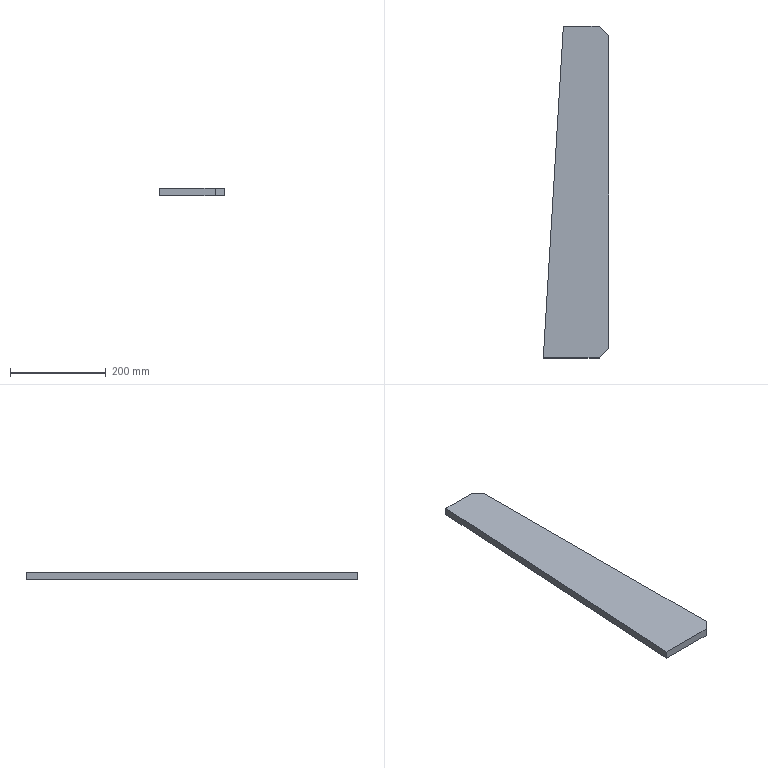Part | SolidWorks | features Chamfer 1, Extrusion 1 | 1 solid | 8 faces | box 137 x 695 x 16 mm | volume 1283520 mm3 | plane 8
STEP:
#1=CARTESIAN_POINT('',(0.,0.,-8.));
#2=VERTEX_POINT('',#1);
#3=CARTESIAN_POINT('',(117.,0.,-8.));
#4=VERTEX_POINT('',#3);
#5=CARTESIAN_POINT('',(137.,0.,-8.));
#6=DIRECTION('',(1.,0.,0.));
#7=VECTOR('',#6,1000.);
#8=LINE('',#5,#7);
#9=EDGE_CURVE('',#2,#4,#8,.T.);
#10=ORIENTED_EDGE('',*,*,#9,.T.);
#11=CARTESIAN_POINT('',(117.,0.,8.));
#12=VERTEX_POINT('',#11);
#13=CARTESIAN_POINT('',(117.,0.,8.));
#14=DIRECTION('',(0.,0.,1.));
#15=VECTOR('',#14,1000.);
#16=LINE('',#13,#15);
#17=EDGE_CURVE('',#4,#12,#16,.T.);
#18=ORIENTED_EDGE('',*,*,#17,.T.);
#19=CARTESIAN_POINT('',(0.,0.,8.));
#20=VERTEX_POINT('',#19);
#21=CARTESIAN_POINT('',(137.,0.,8.));
#22=DIRECTION('',(1.,0.,0.));
#23=VECTOR('',#22,1000.);
#24=LINE('',#21,#23);
#25=EDGE_CURVE('',#20,#12,#24,.T.);
#26=ORIENTED_EDGE('',*,*,#25,.F.);
#27=CARTESIAN_POINT('',(0.,0.,8.));
#28=DIRECTION('',(0.,0.,-1.));
#29=VECTOR('',#28,1000.);
#30=LINE('',#27,#29);
#31=EDGE_CURVE('',#20,#2,#30,.T.);
#32=ORIENTED_EDGE('',*,*,#31,.T.);
#33=EDGE_LOOP('',(#10,#18,#26,#32));
#34=FACE_OUTER_BOUND('',#33,.T.);
#35=CARTESIAN_POINT('',(137.,0.,8.));
#36=DIRECTION('',(0.,1.,0.));
#37=DIRECTION('',(0.,0.,1.));
#38=AXIS2_PLACEMENT_3D('',#35,#36,#37);
#39=PLANE('',#38);
#40=ADVANCED_FACE('',(#34),#39,.F.);
#41=CARTESIAN_POINT('',(137.,20.,8.));
#42=VERTEX_POINT('',#41);
#43=CARTESIAN_POINT('',(137.,675.,8.));
#44=VERTEX_POINT('',#43);
#45=CARTESIAN_POINT('',(137.,695.,8.));
#46=DIRECTION('',(0.,1.,0.));
#47=VECTOR('',#46,1000.);
#48=LINE('',#45,#47);
#49=EDGE_CURVE('',#42,#44,#48,.T.);
#50=ORIENTED_EDGE('',*,*,#49,.F.);
#51=CARTESIAN_POINT('',(137.,20.,-8.));
#52=VERTEX_POINT('',#51);
#53=CARTESIAN_POINT('',(137.,20.,8.));
#54=DIRECTION('',(0.,0.,-1.));
#55=VECTOR('',#54,1000.);
#56=LINE('',#53,#55);
#57=EDGE_CURVE('',#42,#52,#56,.T.);
#58=ORIENTED_EDGE('',*,*,#57,.T.);
#59=CARTESIAN_POINT('',(137.,675.,-8.));
#60=VERTEX_POINT('',#59);
#61=CARTESIAN_POINT('',(137.,695.,-8.));
#62=DIRECTION('',(0.,1.,0.));
#63=VECTOR('',#62,1000.);
#64=LINE('',#61,#63);
#65=EDGE_CURVE('',#52,#60,#64,.T.);
#66=ORIENTED_EDGE('',*,*,#65,.T.);
#67=CARTESIAN_POINT('',(137.,675.,8.));
#68=DIRECTION('',(0.,0.,1.));
#69=VECTOR('',#68,1000.);
#70=LINE('',#67,#69);
#71=EDGE_CURVE('',#60,#44,#70,.T.);
#72=ORIENTED_EDGE('',*,*,#71,.T.);
#73=EDGE_LOOP('',(#50,#58,#66,#72));
#74=FACE_OUTER_BOUND('',#73,.T.);
#75=CARTESIAN_POINT('',(137.,695.,8.));
#76=DIRECTION('',(-1.,0.,0.));
#77=DIRECTION('',(0.,-1.,0.));
#78=AXIS2_PLACEMENT_3D('',#75,#76,#77);
#79=PLANE('',#78);
#80=ADVANCED_FACE('',(#74),#79,.F.);
#81=CARTESIAN_POINT('',(117.,695.,8.));
#82=VERTEX_POINT('',#81);
#83=CARTESIAN_POINT('',(42.,695.,8.));
#84=VERTEX_POINT('',#83);
#85=CARTESIAN_POINT('',(42.,695.,8.));
#86=DIRECTION('',(-1.,0.,0.));
#87=VECTOR('',#86,1000.);
#88=LINE('',#85,#87);
#89=EDGE_CURVE('',#82,#84,#88,.T.);
#90=ORIENTED_EDGE('',*,*,#89,.F.);
#91=CARTESIAN_POINT('',(117.,695.,-8.));
#92=VERTEX_POINT('',#91);
#93=CARTESIAN_POINT('',(117.,695.,8.));
#94=DIRECTION('',(0.,0.,-1.));
#95=VECTOR('',#94,1000.);
#96=LINE('',#93,#95);
#97=EDGE_CURVE('',#82,#92,#96,.T.);
#98=ORIENTED_EDGE('',*,*,#97,.T.);
#99=CARTESIAN_POINT('',(42.,695.,-8.));
#100=VERTEX_POINT('',#99);
#101=CARTESIAN_POINT('',(42.,695.,-8.));
#102=DIRECTION('',(-1.,0.,0.));
#103=VECTOR('',#102,1000.);
#104=LINE('',#101,#103);
#105=EDGE_CURVE('',#92,#100,#104,.T.);
#106=ORIENTED_EDGE('',*,*,#105,.T.);
#107=CARTESIAN_POINT('',(42.,695.,8.));
#108=DIRECTION('',(0.,0.,-1.));
#109=VECTOR('',#108,1000.);
#110=LINE('',#107,#109);
#111=EDGE_CURVE('',#84,#100,#110,.T.);
#112=ORIENTED_EDGE('',*,*,#111,.F.);
#113=EDGE_LOOP('',(#90,#98,#106,#112));
#114=FACE_OUTER_BOUND('',#113,.T.);
#115=CARTESIAN_POINT('',(42.,695.,8.));
#116=DIRECTION('',(0.,-1.,0.));
#117=DIRECTION('',(0.,0.,-1.));
#118=AXIS2_PLACEMENT_3D('',#115,#116,#117);
#119=PLANE('',#118);
#120=ADVANCED_FACE('',(#114),#119,.F.);
#121=CARTESIAN_POINT('',(0.,0.,-8.));
#122=DIRECTION('',(-0.06032,-0.9982,0.));
#123=VECTOR('',#122,1000.);
#124=LINE('',#121,#123);
#125=EDGE_CURVE('',#100,#2,#124,.T.);
#126=ORIENTED_EDGE('',*,*,#125,.T.);
#127=ORIENTED_EDGE('',*,*,#31,.F.);
#128=CARTESIAN_POINT('',(0.,0.,8.));
#129=DIRECTION('',(-0.06032,-0.9982,0.));
#130=VECTOR('',#129,1000.);
#131=LINE('',#128,#130);
#132=EDGE_CURVE('',#84,#20,#131,.T.);
#133=ORIENTED_EDGE('',*,*,#132,.F.);
#134=ORIENTED_EDGE('',*,*,#111,.T.);
#135=EDGE_LOOP('',(#126,#127,#133,#134));
#136=FACE_OUTER_BOUND('',#135,.T.);
#137=CARTESIAN_POINT('',(0.,0.,8.));
#138=DIRECTION('',(0.9982,-0.06032,0.));
#139=DIRECTION('',(0.06032,0.9982,0.));
#140=AXIS2_PLACEMENT_3D('',#137,#138,#139);
#141=PLANE('',#140);
#142=ADVANCED_FACE('',(#136),#141,.F.);
#143=ORIENTED_EDGE('',*,*,#25,.T.);
#144=CARTESIAN_POINT('',(58.5,-58.5,8.));
#145=DIRECTION('',(0.7071,0.7071,0.));
#146=VECTOR('',#145,1000.);
#147=LINE('',#144,#146);
#148=EDGE_CURVE('',#12,#42,#147,.T.);
#149=ORIENTED_EDGE('',*,*,#148,.T.);
#150=ORIENTED_EDGE('',*,*,#49,.T.);
#151=CARTESIAN_POINT('',(406.,406.,8.));
#152=DIRECTION('',(-0.7071,0.7071,0.));
#153=VECTOR('',#152,1000.);
#154=LINE('',#151,#153);
#155=EDGE_CURVE('',#44,#82,#154,.T.);
#156=ORIENTED_EDGE('',*,*,#155,.T.);
#157=ORIENTED_EDGE('',*,*,#89,.T.);
#158=ORIENTED_EDGE('',*,*,#132,.T.);
#159=EDGE_LOOP('',(#143,#149,#150,#156,#157,#158));
#160=FACE_OUTER_BOUND('',#159,.T.);
#161=CARTESIAN_POINT('',(0.,0.,8.));
#162=DIRECTION('',(0.,0.,1.));
#163=DIRECTION('',(1.,0.,0.));
#164=AXIS2_PLACEMENT_3D('',#161,#162,#163);
#165=PLANE('',#164);
#166=ADVANCED_FACE('',(#160),#165,.T.);
#167=ORIENTED_EDGE('',*,*,#65,.F.);
#168=CARTESIAN_POINT('',(137.,20.,-8.));
#169=DIRECTION('',(-0.7071,-0.7071,0.));
#170=VECTOR('',#169,1000.);
#171=LINE('',#168,#170);
#172=EDGE_CURVE('',#52,#4,#171,.T.);
#173=ORIENTED_EDGE('',*,*,#172,.T.);
#174=ORIENTED_EDGE('',*,*,#9,.F.);
#175=ORIENTED_EDGE('',*,*,#125,.F.);
#176=ORIENTED_EDGE('',*,*,#105,.F.);
#177=CARTESIAN_POINT('',(117.,695.,-8.));
#178=DIRECTION('',(0.7071,-0.7071,0.));
#179=VECTOR('',#178,1000.);
#180=LINE('',#177,#179);
#181=EDGE_CURVE('',#92,#60,#180,.T.);
#182=ORIENTED_EDGE('',*,*,#181,.T.);
#183=EDGE_LOOP('',(#167,#173,#174,#175,#176,#182));
#184=FACE_OUTER_BOUND('',#183,.T.);
#185=CARTESIAN_POINT('',(0.,0.,-8.));
#186=DIRECTION('',(0.,0.,1.));
#187=DIRECTION('',(1.,0.,0.));
#188=AXIS2_PLACEMENT_3D('',#185,#186,#187);
#189=PLANE('',#188);
#190=ADVANCED_FACE('',(#184),#189,.F.);
#191=ORIENTED_EDGE('',*,*,#148,.F.);
#192=ORIENTED_EDGE('',*,*,#17,.F.);
#193=ORIENTED_EDGE('',*,*,#172,.F.);
#194=ORIENTED_EDGE('',*,*,#57,.F.);
#195=EDGE_LOOP('',(#191,#192,#193,#194));
#196=FACE_OUTER_BOUND('',#195,.T.);
#197=CARTESIAN_POINT('',(137.,20.,8.));
#198=DIRECTION('',(-0.7071,0.7071,0.));
#199=DIRECTION('',(0.,0.,-1.));
#200=AXIS2_PLACEMENT_3D('',#197,#198,#199);
#201=PLANE('',#200);
#202=ADVANCED_FACE('',(#196),#201,.F.);
#203=ORIENTED_EDGE('',*,*,#155,.F.);
#204=ORIENTED_EDGE('',*,*,#71,.F.);
#205=ORIENTED_EDGE('',*,*,#181,.F.);
#206=ORIENTED_EDGE('',*,*,#97,.F.);
#207=EDGE_LOOP('',(#203,#204,#205,#206));
#208=FACE_OUTER_BOUND('',#207,.T.);
#209=CARTESIAN_POINT('',(117.,695.,8.));
#210=DIRECTION('',(-0.7071,-0.7071,0.));
#211=DIRECTION('',(0.,0.,-1.));
#212=AXIS2_PLACEMENT_3D('',#209,#210,#211);
#213=PLANE('',#212);
#214=ADVANCED_FACE('',(#208),#213,.F.);
#215=CLOSED_SHELL('',(#40,#80,#120,#142,#166,#190,#202,#214));
#216=MANIFOLD_SOLID_BREP('',#215);
#217=CARTESIAN_POINT('',(0.,0.,0.));
#218=DIRECTION('',(0.,0.,1.));
#219=DIRECTION('',(1.,0.,0.));
#220=AXIS2_PLACEMENT_3D('',#217,#218,#219);
#221=(LENGTH_UNIT()NAMED_UNIT(*)SI_UNIT(.MILLI.,.METRE.));
#222=UNCERTAINTY_MEASURE_WITH_UNIT(LENGTH_MEASURE(0.00001),#221,'','');
#223=(NAMED_UNIT(*)PLANE_ANGLE_UNIT()SI_UNIT($,.RADIAN.));
#224=(NAMED_UNIT(*)SI_UNIT($,.STERADIAN.)SOLID_ANGLE_UNIT());
#225=(GEOMETRIC_REPRESENTATION_CONTEXT(3)GLOBAL_UNCERTAINTY_ASSIGNED_CONTEXT((#222))GLOBAL_UNIT_ASSIGNED_CONTEXT((#221,#223,#224))REPRESENTATION_CONTEXT('',''));
#226=ADVANCED_BREP_SHAPE_REPRESENTATION('',(#216,#220),#225);